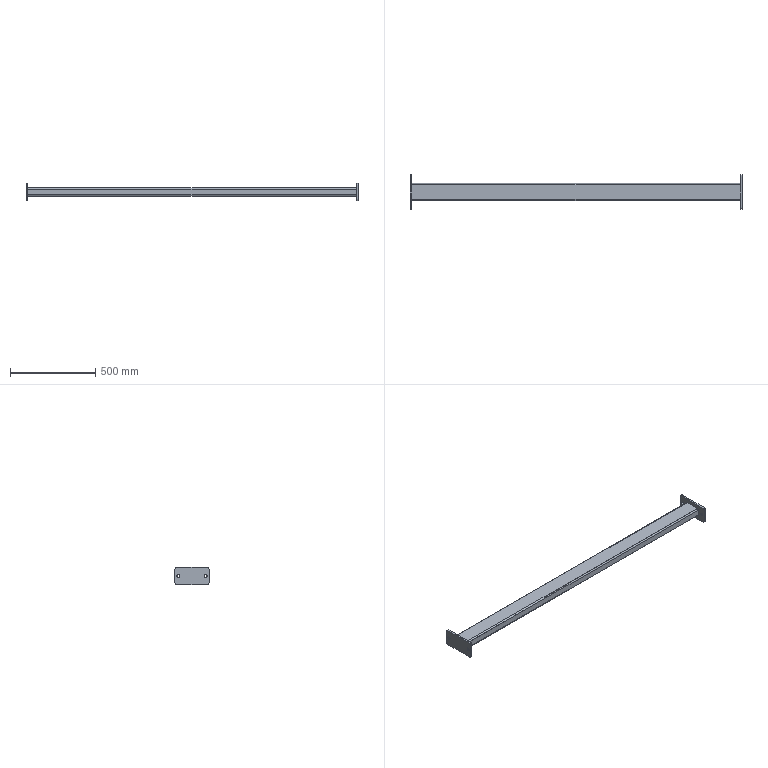Part | SolidWorks | features Fillet 1, HoleWzd 1, ICE 1, MirrorSolid 1, WeldMemberFeat 1, WeldmentFeature 1 | 3 solids | 46 faces | box 1950 x 200 x 100 mm | volume 2501619 mm3 | cylinder 24 | plane 22 | commonest cylinder face diameters 17.5 x8 20 x8 8 x4 16 x4
STEP:
#1=CARTESIAN_POINT('',(-965.,42.,-25.));
#2=VERTEX_POINT('',#1);
#3=CARTESIAN_POINT('',(-965.,50.,-17.));
#4=VERTEX_POINT('',#3);
#5=CARTESIAN_POINT('',(-965.,42.,-17.));
#6=DIRECTION('',(1.,0.,0.));
#7=DIRECTION('',(0.,0.,-1.));
#8=AXIS2_PLACEMENT_3D('',#5,#6,#7);
#9=CIRCLE('',#8,8.);
#10=EDGE_CURVE('',#2,#4,#9,.T.);
#11=ORIENTED_EDGE('',*,*,#10,.T.);
#12=CARTESIAN_POINT('',(965.,50.,-17.));
#13=VERTEX_POINT('',#12);
#14=CARTESIAN_POINT('',(965.,50.,-17.));
#15=DIRECTION('',(-1.,0.,0.));
#16=VECTOR('',#15,1000.);
#17=LINE('',#14,#16);
#18=EDGE_CURVE('',#13,#4,#17,.T.);
#19=ORIENTED_EDGE('',*,*,#18,.F.);
#20=CARTESIAN_POINT('',(965.,42.,-25.));
#21=VERTEX_POINT('',#20);
#22=CARTESIAN_POINT('',(965.,42.,-17.));
#23=DIRECTION('',(1.,0.,0.));
#24=DIRECTION('',(0.,0.,-1.));
#25=AXIS2_PLACEMENT_3D('',#22,#23,#24);
#26=CIRCLE('',#25,8.);
#27=EDGE_CURVE('',#21,#13,#26,.T.);
#28=ORIENTED_EDGE('',*,*,#27,.F.);
#29=CARTESIAN_POINT('',(965.,42.,-25.));
#30=DIRECTION('',(-1.,0.,0.));
#31=VECTOR('',#30,1000.);
#32=LINE('',#29,#31);
#33=EDGE_CURVE('',#21,#2,#32,.T.);
#34=ORIENTED_EDGE('',*,*,#33,.T.);
#35=EDGE_LOOP('',(#11,#19,#28,#34));
#36=FACE_OUTER_BOUND('',#35,.T.);
#37=CARTESIAN_POINT('',(965.,42.,-17.));
#38=DIRECTION('',(-1.,0.,0.));
#39=DIRECTION('',(0.,0.,1.));
#40=AXIS2_PLACEMENT_3D('',#37,#38,#39);
#41=CYLINDRICAL_SURFACE('',#40,8.);
#42=ADVANCED_FACE('',(#36),#41,.T.);
#43=CARTESIAN_POINT('',(-965.,50.,17.));
#44=VERTEX_POINT('',#43);
#45=CARTESIAN_POINT('',(-965.,50.,-17.));
#46=DIRECTION('',(0.,0.,1.));
#47=VECTOR('',#46,1000.);
#48=LINE('',#45,#47);
#49=EDGE_CURVE('',#4,#44,#48,.T.);
#50=ORIENTED_EDGE('',*,*,#49,.T.);
#51=CARTESIAN_POINT('',(965.,50.,17.));
#52=VERTEX_POINT('',#51);
#53=CARTESIAN_POINT('',(965.,50.,17.));
#54=DIRECTION('',(-1.,0.,0.));
#55=VECTOR('',#54,1000.);
#56=LINE('',#53,#55);
#57=EDGE_CURVE('',#52,#44,#56,.T.);
#58=ORIENTED_EDGE('',*,*,#57,.F.);
#59=CARTESIAN_POINT('',(965.,50.,-17.));
#60=DIRECTION('',(0.,0.,1.));
#61=VECTOR('',#60,1000.);
#62=LINE('',#59,#61);
#63=EDGE_CURVE('',#13,#52,#62,.T.);
#64=ORIENTED_EDGE('',*,*,#63,.F.);
#65=ORIENTED_EDGE('',*,*,#18,.T.);
#66=EDGE_LOOP('',(#50,#58,#64,#65));
#67=FACE_OUTER_BOUND('',#66,.T.);
#68=CARTESIAN_POINT('',(965.,50.,-17.));
#69=DIRECTION('',(0.,-1.,0.));
#70=DIRECTION('',(0.,0.,-1.));
#71=AXIS2_PLACEMENT_3D('',#68,#69,#70);
#72=PLANE('',#71);
#73=ADVANCED_FACE('',(#67),#72,.F.);
#74=CARTESIAN_POINT('',(-965.,42.,25.));
#75=VERTEX_POINT('',#74);
#76=CARTESIAN_POINT('',(-965.,42.,17.));
#77=DIRECTION('',(1.,0.,0.));
#78=DIRECTION('',(0.,0.,-1.));
#79=AXIS2_PLACEMENT_3D('',#76,#77,#78);
#80=CIRCLE('',#79,8.);
#81=EDGE_CURVE('',#44,#75,#80,.T.);
#82=ORIENTED_EDGE('',*,*,#81,.T.);
#83=CARTESIAN_POINT('',(965.,42.,25.));
#84=VERTEX_POINT('',#83);
#85=CARTESIAN_POINT('',(965.,42.,25.));
#86=DIRECTION('',(-1.,0.,0.));
#87=VECTOR('',#86,1000.);
#88=LINE('',#85,#87);
#89=EDGE_CURVE('',#84,#75,#88,.T.);
#90=ORIENTED_EDGE('',*,*,#89,.F.);
#91=CARTESIAN_POINT('',(965.,42.,17.));
#92=DIRECTION('',(1.,0.,0.));
#93=DIRECTION('',(0.,0.,-1.));
#94=AXIS2_PLACEMENT_3D('',#91,#92,#93);
#95=CIRCLE('',#94,8.);
#96=EDGE_CURVE('',#52,#84,#95,.T.);
#97=ORIENTED_EDGE('',*,*,#96,.F.);
#98=ORIENTED_EDGE('',*,*,#57,.T.);
#99=EDGE_LOOP('',(#82,#90,#97,#98));
#100=FACE_OUTER_BOUND('',#99,.T.);
#101=CARTESIAN_POINT('',(965.,42.,17.));
#102=DIRECTION('',(-1.,0.,0.));
#103=DIRECTION('',(0.,0.,1.));
#104=AXIS2_PLACEMENT_3D('',#101,#102,#103);
#105=CYLINDRICAL_SURFACE('',#104,8.);
#106=ADVANCED_FACE('',(#100),#105,.T.);
#107=CARTESIAN_POINT('',(-965.,-42.,25.));
#108=VERTEX_POINT('',#107);
#109=CARTESIAN_POINT('',(-965.,-42.,25.));
#110=DIRECTION('',(0.,-1.,0.));
#111=VECTOR('',#110,1000.);
#112=LINE('',#109,#111);
#113=EDGE_CURVE('',#75,#108,#112,.T.);
#114=ORIENTED_EDGE('',*,*,#113,.T.);
#115=CARTESIAN_POINT('',(965.,-42.,25.));
#116=VERTEX_POINT('',#115);
#117=CARTESIAN_POINT('',(965.,-42.,25.));
#118=DIRECTION('',(-1.,0.,0.));
#119=VECTOR('',#118,1000.);
#120=LINE('',#117,#119);
#121=EDGE_CURVE('',#116,#108,#120,.T.);
#122=ORIENTED_EDGE('',*,*,#121,.F.);
#123=CARTESIAN_POINT('',(965.,-42.,25.));
#124=DIRECTION('',(0.,-1.,0.));
#125=VECTOR('',#124,1000.);
#126=LINE('',#123,#125);
#127=EDGE_CURVE('',#84,#116,#126,.T.);
#128=ORIENTED_EDGE('',*,*,#127,.F.);
#129=ORIENTED_EDGE('',*,*,#89,.T.);
#130=EDGE_LOOP('',(#114,#122,#128,#129));
#131=FACE_OUTER_BOUND('',#130,.T.);
#132=CARTESIAN_POINT('',(965.,-42.,25.));
#133=DIRECTION('',(0.,0.,-1.));
#134=DIRECTION('',(-1.,0.,0.));
#135=AXIS2_PLACEMENT_3D('',#132,#133,#134);
#136=PLANE('',#135);
#137=ADVANCED_FACE('',(#131),#136,.F.);
#138=CARTESIAN_POINT('',(-965.,-50.,17.));
#139=VERTEX_POINT('',#138);
#140=CARTESIAN_POINT('',(-965.,-42.,17.));
#141=DIRECTION('',(1.,0.,0.));
#142=DIRECTION('',(0.,0.,-1.));
#143=AXIS2_PLACEMENT_3D('',#140,#141,#142);
#144=CIRCLE('',#143,8.);
#145=EDGE_CURVE('',#108,#139,#144,.T.);
#146=ORIENTED_EDGE('',*,*,#145,.T.);
#147=CARTESIAN_POINT('',(965.,-50.,17.));
#148=VERTEX_POINT('',#147);
#149=CARTESIAN_POINT('',(965.,-50.,17.));
#150=DIRECTION('',(-1.,0.,0.));
#151=VECTOR('',#150,1000.);
#152=LINE('',#149,#151);
#153=EDGE_CURVE('',#148,#139,#152,.T.);
#154=ORIENTED_EDGE('',*,*,#153,.F.);
#155=CARTESIAN_POINT('',(965.,-42.,17.));
#156=DIRECTION('',(1.,0.,0.));
#157=DIRECTION('',(0.,0.,-1.));
#158=AXIS2_PLACEMENT_3D('',#155,#156,#157);
#159=CIRCLE('',#158,8.);
#160=EDGE_CURVE('',#116,#148,#159,.T.);
#161=ORIENTED_EDGE('',*,*,#160,.F.);
#162=ORIENTED_EDGE('',*,*,#121,.T.);
#163=EDGE_LOOP('',(#146,#154,#161,#162));
#164=FACE_OUTER_BOUND('',#163,.T.);
#165=CARTESIAN_POINT('',(965.,-42.,17.));
#166=DIRECTION('',(-1.,0.,0.));
#167=DIRECTION('',(0.,0.,1.));
#168=AXIS2_PLACEMENT_3D('',#165,#166,#167);
#169=CYLINDRICAL_SURFACE('',#168,8.);
#170=ADVANCED_FACE('',(#164),#169,.T.);
#171=CARTESIAN_POINT('',(-965.,-50.,-17.));
#172=VERTEX_POINT('',#171);
#173=CARTESIAN_POINT('',(-965.,-50.,17.));
#174=DIRECTION('',(0.,0.,-1.));
#175=VECTOR('',#174,1000.);
#176=LINE('',#173,#175);
#177=EDGE_CURVE('',#139,#172,#176,.T.);
#178=ORIENTED_EDGE('',*,*,#177,.T.);
#179=CARTESIAN_POINT('',(965.,-50.,-17.));
#180=VERTEX_POINT('',#179);
#181=CARTESIAN_POINT('',(965.,-50.,-17.));
#182=DIRECTION('',(-1.,0.,0.));
#183=VECTOR('',#182,1000.);
#184=LINE('',#181,#183);
#185=EDGE_CURVE('',#180,#172,#184,.T.);
#186=ORIENTED_EDGE('',*,*,#185,.F.);
#187=CARTESIAN_POINT('',(965.,-50.,17.));
#188=DIRECTION('',(0.,0.,-1.));
#189=VECTOR('',#188,1000.);
#190=LINE('',#187,#189);
#191=EDGE_CURVE('',#148,#180,#190,.T.);
#192=ORIENTED_EDGE('',*,*,#191,.F.);
#193=ORIENTED_EDGE('',*,*,#153,.T.);
#194=EDGE_LOOP('',(#178,#186,#192,#193));
#195=FACE_OUTER_BOUND('',#194,.T.);
#196=CARTESIAN_POINT('',(965.,-50.,17.));
#197=DIRECTION('',(0.,1.,0.));
#198=DIRECTION('',(0.,0.,1.));
#199=AXIS2_PLACEMENT_3D('',#196,#197,#198);
#200=PLANE('',#199);
#201=ADVANCED_FACE('',(#195),#200,.F.);
#202=CARTESIAN_POINT('',(-965.,-42.,-25.));
#203=VERTEX_POINT('',#202);
#204=CARTESIAN_POINT('',(-965.,-42.,-17.));
#205=DIRECTION('',(1.,0.,0.));
#206=DIRECTION('',(0.,0.,-1.));
#207=AXIS2_PLACEMENT_3D('',#204,#205,#206);
#208=CIRCLE('',#207,8.);
#209=EDGE_CURVE('',#172,#203,#208,.T.);
#210=ORIENTED_EDGE('',*,*,#209,.T.);
#211=CARTESIAN_POINT('',(965.,-42.,-25.));
#212=VERTEX_POINT('',#211);
#213=CARTESIAN_POINT('',(965.,-42.,-25.));
#214=DIRECTION('',(-1.,0.,0.));
#215=VECTOR('',#214,1000.);
#216=LINE('',#213,#215);
#217=EDGE_CURVE('',#212,#203,#216,.T.);
#218=ORIENTED_EDGE('',*,*,#217,.F.);
#219=CARTESIAN_POINT('',(965.,-42.,-17.));
#220=DIRECTION('',(1.,0.,0.));
#221=DIRECTION('',(0.,0.,-1.));
#222=AXIS2_PLACEMENT_3D('',#219,#220,#221);
#223=CIRCLE('',#222,8.);
#224=EDGE_CURVE('',#180,#212,#223,.T.);
#225=ORIENTED_EDGE('',*,*,#224,.F.);
#226=ORIENTED_EDGE('',*,*,#185,.T.);
#227=EDGE_LOOP('',(#210,#218,#225,#226));
#228=FACE_OUTER_BOUND('',#227,.T.);
#229=CARTESIAN_POINT('',(965.,-42.,-17.));
#230=DIRECTION('',(-1.,0.,0.));
#231=DIRECTION('',(0.,0.,1.));
#232=AXIS2_PLACEMENT_3D('',#229,#230,#231);
#233=CYLINDRICAL_SURFACE('',#232,8.);
#234=ADVANCED_FACE('',(#228),#233,.T.);
#235=CARTESIAN_POINT('',(-965.,46.,17.));
#236=VERTEX_POINT('',#235);
#237=CARTESIAN_POINT('',(-965.,42.,21.));
#238=VERTEX_POINT('',#237);
#239=CARTESIAN_POINT('',(-965.,42.,17.));
#240=DIRECTION('',(1.,0.,0.));
#241=DIRECTION('',(0.,0.,-1.));
#242=AXIS2_PLACEMENT_3D('',#239,#240,#241);
#243=CIRCLE('',#242,4.);
#244=EDGE_CURVE('',#236,#238,#243,.T.);
#245=ORIENTED_EDGE('',*,*,#244,.F.);
#246=CARTESIAN_POINT('',(965.,46.,17.));
#247=VERTEX_POINT('',#246);
#248=CARTESIAN_POINT('',(965.,46.,17.));
#249=DIRECTION('',(-1.,0.,0.));
#250=VECTOR('',#249,1000.);
#251=LINE('',#248,#250);
#252=EDGE_CURVE('',#247,#236,#251,.T.);
#253=ORIENTED_EDGE('',*,*,#252,.F.);
#254=CARTESIAN_POINT('',(965.,42.,21.));
#255=VERTEX_POINT('',#254);
#256=CARTESIAN_POINT('',(965.,42.,17.));
#257=DIRECTION('',(1.,0.,0.));
#258=DIRECTION('',(0.,0.,-1.));
#259=AXIS2_PLACEMENT_3D('',#256,#257,#258);
#260=CIRCLE('',#259,4.);
#261=EDGE_CURVE('',#247,#255,#260,.T.);
#262=ORIENTED_EDGE('',*,*,#261,.T.);
#263=CARTESIAN_POINT('',(965.,42.,21.));
#264=DIRECTION('',(-1.,0.,0.));
#265=VECTOR('',#264,1000.);
#266=LINE('',#263,#265);
#267=EDGE_CURVE('',#255,#238,#266,.T.);
#268=ORIENTED_EDGE('',*,*,#267,.T.);
#269=EDGE_LOOP('',(#245,#253,#262,#268));
#270=FACE_OUTER_BOUND('',#269,.T.);
#271=CARTESIAN_POINT('',(965.,42.,17.));
#272=DIRECTION('',(-1.,0.,0.));
#273=DIRECTION('',(0.,0.,1.));
#274=AXIS2_PLACEMENT_3D('',#271,#272,#273);
#275=CYLINDRICAL_SURFACE('',#274,4.);
#276=ADVANCED_FACE('',(#270),#275,.F.);
#277=CARTESIAN_POINT('',(-965.,46.,-17.));
#278=VERTEX_POINT('',#277);
#279=CARTESIAN_POINT('',(-965.,46.,-17.));
#280=DIRECTION('',(0.,0.,1.));
#281=VECTOR('',#280,1000.);
#282=LINE('',#279,#281);
#283=EDGE_CURVE('',#278,#236,#282,.T.);
#284=ORIENTED_EDGE('',*,*,#283,.F.);
#285=CARTESIAN_POINT('',(965.,46.,-17.));
#286=VERTEX_POINT('',#285);
#287=CARTESIAN_POINT('',(965.,46.,-17.));
#288=DIRECTION('',(-1.,0.,0.));
#289=VECTOR('',#288,1000.);
#290=LINE('',#287,#289);
#291=EDGE_CURVE('',#286,#278,#290,.T.);
#292=ORIENTED_EDGE('',*,*,#291,.F.);
#293=CARTESIAN_POINT('',(965.,46.,-17.));
#294=DIRECTION('',(0.,0.,1.));
#295=VECTOR('',#294,1000.);
#296=LINE('',#293,#295);
#297=EDGE_CURVE('',#286,#247,#296,.T.);
#298=ORIENTED_EDGE('',*,*,#297,.T.);
#299=ORIENTED_EDGE('',*,*,#252,.T.);
#300=EDGE_LOOP('',(#284,#292,#298,#299));
#301=FACE_OUTER_BOUND('',#300,.T.);
#302=CARTESIAN_POINT('',(965.,46.,-17.));
#303=DIRECTION('',(0.,-1.,0.));
#304=DIRECTION('',(0.,0.,-1.));
#305=AXIS2_PLACEMENT_3D('',#302,#303,#304);
#306=PLANE('',#305);
#307=ADVANCED_FACE('',(#301),#306,.T.);
#308=CARTESIAN_POINT('',(-965.,42.,-21.));
#309=VERTEX_POINT('',#308);
#310=CARTESIAN_POINT('',(-965.,42.,-17.));
#311=DIRECTION('',(1.,0.,0.));
#312=DIRECTION('',(0.,0.,-1.));
#313=AXIS2_PLACEMENT_3D('',#310,#311,#312);
#314=CIRCLE('',#313,4.);
#315=EDGE_CURVE('',#309,#278,#314,.T.);
#316=ORIENTED_EDGE('',*,*,#315,.F.);
#317=CARTESIAN_POINT('',(965.,42.,-21.));
#318=VERTEX_POINT('',#317);
#319=CARTESIAN_POINT('',(965.,42.,-21.));
#320=DIRECTION('',(-1.,0.,0.));
#321=VECTOR('',#320,1000.);
#322=LINE('',#319,#321);
#323=EDGE_CURVE('',#318,#309,#322,.T.);
#324=ORIENTED_EDGE('',*,*,#323,.F.);
#325=CARTESIAN_POINT('',(965.,42.,-17.));
#326=DIRECTION('',(1.,0.,0.));
#327=DIRECTION('',(0.,0.,-1.));
#328=AXIS2_PLACEMENT_3D('',#325,#326,#327);
#329=CIRCLE('',#328,4.);
#330=EDGE_CURVE('',#318,#286,#329,.T.);
#331=ORIENTED_EDGE('',*,*,#330,.T.);
#332=ORIENTED_EDGE('',*,*,#291,.T.);
#333=EDGE_LOOP('',(#316,#324,#331,#332));
#334=FACE_OUTER_BOUND('',#333,.T.);
#335=CARTESIAN_POINT('',(965.,42.,-17.));
#336=DIRECTION('',(-1.,0.,0.));
#337=DIRECTION('',(0.,0.,1.));
#338=AXIS2_PLACEMENT_3D('',#335,#336,#337);
#339=CYLINDRICAL_SURFACE('',#338,4.);
#340=ADVANCED_FACE('',(#334),#339,.F.);
#341=CARTESIAN_POINT('',(-965.,-42.,-21.));
#342=VERTEX_POINT('',#341);
#343=CARTESIAN_POINT('',(-965.,42.,-21.));
#344=DIRECTION('',(0.,1.,0.));
#345=VECTOR('',#344,1000.);
#346=LINE('',#343,#345);
#347=EDGE_CURVE('',#342,#309,#346,.T.);
#348=ORIENTED_EDGE('',*,*,#347,.F.);
#349=CARTESIAN_POINT('',(965.,-42.,-21.));
#350=VERTEX_POINT('',#349);
#351=CARTESIAN_POINT('',(965.,-42.,-21.));
#352=DIRECTION('',(-1.,0.,0.));
#353=VECTOR('',#352,1000.);
#354=LINE('',#351,#353);
#355=EDGE_CURVE('',#350,#342,#354,.T.);
#356=ORIENTED_EDGE('',*,*,#355,.F.);
#357=CARTESIAN_POINT('',(965.,42.,-21.));
#358=DIRECTION('',(0.,1.,0.));
#359=VECTOR('',#358,1000.);
#360=LINE('',#357,#359);
#361=EDGE_CURVE('',#350,#318,#360,.T.);
#362=ORIENTED_EDGE('',*,*,#361,.T.);
#363=ORIENTED_EDGE('',*,*,#323,.T.);
#364=EDGE_LOOP('',(#348,#356,#362,#363));
#365=FACE_OUTER_BOUND('',#364,.T.);
#366=CARTESIAN_POINT('',(965.,42.,-21.));
#367=DIRECTION('',(0.,0.,1.));
#368=DIRECTION('',(1.,0.,0.));
#369=AXIS2_PLACEMENT_3D('',#366,#367,#368);
#370=PLANE('',#369);
#371=ADVANCED_FACE('',(#365),#370,.T.);
#372=CARTESIAN_POINT('',(-965.,-46.,-17.));
#373=VERTEX_POINT('',#372);
#374=CARTESIAN_POINT('',(-965.,-42.,-17.));
#375=DIRECTION('',(1.,0.,0.));
#376=DIRECTION('',(0.,0.,-1.));
#377=AXIS2_PLACEMENT_3D('',#374,#375,#376);
#378=CIRCLE('',#377,4.);
#379=EDGE_CURVE('',#373,#342,#378,.T.);
#380=ORIENTED_EDGE('',*,*,#379,.F.);
#381=CARTESIAN_POINT('',(965.,-46.,-17.));
#382=VERTEX_POINT('',#381);
#383=CARTESIAN_POINT('',(965.,-46.,-17.));
#384=DIRECTION('',(-1.,0.,0.));
#385=VECTOR('',#384,1000.);
#386=LINE('',#383,#385);
#387=EDGE_CURVE('',#382,#373,#386,.T.);
#388=ORIENTED_EDGE('',*,*,#387,.F.);
#389=CARTESIAN_POINT('',(965.,-42.,-17.));
#390=DIRECTION('',(1.,0.,0.));
#391=DIRECTION('',(0.,0.,-1.));
#392=AXIS2_PLACEMENT_3D('',#389,#390,#391);
#393=CIRCLE('',#392,4.);
#394=EDGE_CURVE('',#382,#350,#393,.T.);
#395=ORIENTED_EDGE('',*,*,#394,.T.);
#396=ORIENTED_EDGE('',*,*,#355,.T.);
#397=EDGE_LOOP('',(#380,#388,#395,#396));
#398=FACE_OUTER_BOUND('',#397,.T.);
#399=CARTESIAN_POINT('',(965.,-42.,-17.));
#400=DIRECTION('',(-1.,0.,0.));
#401=DIRECTION('',(0.,0.,1.));
#402=AXIS2_PLACEMENT_3D('',#399,#400,#401);
#403=CYLINDRICAL_SURFACE('',#402,4.);
#404=ADVANCED_FACE('',(#398),#403,.F.);
#405=CARTESIAN_POINT('',(-965.,-46.,17.));
#406=VERTEX_POINT('',#405);
#407=CARTESIAN_POINT('',(-965.,-46.,17.));
#408=DIRECTION('',(0.,0.,-1.));
#409=VECTOR('',#408,1000.);
#410=LINE('',#407,#409);
#411=EDGE_CURVE('',#406,#373,#410,.T.);
#412=ORIENTED_EDGE('',*,*,#411,.F.);
#413=CARTESIAN_POINT('',(965.,-46.,17.));
#414=VERTEX_POINT('',#413);
#415=CARTESIAN_POINT('',(965.,-46.,17.));
#416=DIRECTION('',(-1.,0.,0.));
#417=VECTOR('',#416,1000.);
#418=LINE('',#415,#417);
#419=EDGE_CURVE('',#414,#406,#418,.T.);
#420=ORIENTED_EDGE('',*,*,#419,.F.);
#421=CARTESIAN_POINT('',(965.,-46.,17.));
#422=DIRECTION('',(0.,0.,-1.));
#423=VECTOR('',#422,1000.);
#424=LINE('',#421,#423);
#425=EDGE_CURVE('',#414,#382,#424,.T.);
#426=ORIENTED_EDGE('',*,*,#425,.T.);
#427=ORIENTED_EDGE('',*,*,#387,.T.);
#428=EDGE_LOOP('',(#412,#420,#426,#427));
#429=FACE_OUTER_BOUND('',#428,.T.);
#430=CARTESIAN_POINT('',(965.,-46.,17.));
#431=DIRECTION('',(0.,1.,0.));
#432=DIRECTION('',(0.,0.,1.));
#433=AXIS2_PLACEMENT_3D('',#430,#431,#432);
#434=PLANE('',#433);
#435=ADVANCED_FACE('',(#429),#434,.T.);
#436=CARTESIAN_POINT('',(-965.,-42.,21.));
#437=VERTEX_POINT('',#436);
#438=CARTESIAN_POINT('',(-965.,-42.,17.));
#439=DIRECTION('',(1.,0.,0.));
#440=DIRECTION('',(0.,0.,-1.));
#441=AXIS2_PLACEMENT_3D('',#438,#439,#440);
#442=CIRCLE('',#441,4.);
#443=EDGE_CURVE('',#437,#406,#442,.T.);
#444=ORIENTED_EDGE('',*,*,#443,.F.);
#445=CARTESIAN_POINT('',(965.,-42.,21.));
#446=VERTEX_POINT('',#445);
#447=CARTESIAN_POINT('',(965.,-42.,21.));
#448=DIRECTION('',(-1.,0.,0.));
#449=VECTOR('',#448,1000.);
#450=LINE('',#447,#449);
#451=EDGE_CURVE('',#446,#437,#450,.T.);
#452=ORIENTED_EDGE('',*,*,#451,.F.);
#453=CARTESIAN_POINT('',(965.,-42.,17.));
#454=DIRECTION('',(1.,0.,0.));
#455=DIRECTION('',(0.,0.,-1.));
#456=AXIS2_PLACEMENT_3D('',#453,#454,#455);
#457=CIRCLE('',#456,4.);
#458=EDGE_CURVE('',#446,#414,#457,.T.);
#459=ORIENTED_EDGE('',*,*,#458,.T.);
#460=ORIENTED_EDGE('',*,*,#419,.T.);
#461=EDGE_LOOP('',(#444,#452,#459,#460));
#462=FACE_OUTER_BOUND('',#461,.T.);
#463=CARTESIAN_POINT('',(965.,-42.,17.));
#464=DIRECTION('',(-1.,0.,0.));
#465=DIRECTION('',(0.,0.,1.));
#466=AXIS2_PLACEMENT_3D('',#463,#464,#465);
#467=CYLINDRICAL_SURFACE('',#466,4.);
#468=ADVANCED_FACE('',(#462),#467,.F.);
#469=CARTESIAN_POINT('',(-965.,-42.,21.));
#470=DIRECTION('',(0.,-1.,0.));
#471=VECTOR('',#470,1000.);
#472=LINE('',#469,#471);
#473=EDGE_CURVE('',#238,#437,#472,.T.);
#474=ORIENTED_EDGE('',*,*,#473,.F.);
#475=ORIENTED_EDGE('',*,*,#267,.F.);
#476=CARTESIAN_POINT('',(965.,-42.,21.));
#477=DIRECTION('',(0.,-1.,0.));
#478=VECTOR('',#477,1000.);
#479=LINE('',#476,#478);
#480=EDGE_CURVE('',#255,#446,#479,.T.);
#481=ORIENTED_EDGE('',*,*,#480,.T.);
#482=ORIENTED_EDGE('',*,*,#451,.T.);
#483=EDGE_LOOP('',(#474,#475,#481,#482));
#484=FACE_OUTER_BOUND('',#483,.T.);
#485=CARTESIAN_POINT('',(965.,-42.,21.));
#486=DIRECTION('',(0.,0.,-1.));
#487=DIRECTION('',(-1.,0.,0.));
#488=AXIS2_PLACEMENT_3D('',#485,#486,#487);
#489=PLANE('',#488);
#490=ADVANCED_FACE('',(#484),#489,.T.);
#491=CARTESIAN_POINT('',(-965.,42.,-25.));
#492=DIRECTION('',(0.,1.,0.));
#493=VECTOR('',#492,1000.);
#494=LINE('',#491,#493);
#495=EDGE_CURVE('',#203,#2,#494,.T.);
#496=ORIENTED_EDGE('',*,*,#495,.T.);
#497=ORIENTED_EDGE('',*,*,#33,.F.);
#498=CARTESIAN_POINT('',(965.,42.,-25.));
#499=DIRECTION('',(0.,1.,0.));
#500=VECTOR('',#499,1000.);
#501=LINE('',#498,#500);
#502=EDGE_CURVE('',#212,#21,#501,.T.);
#503=ORIENTED_EDGE('',*,*,#502,.F.);
#504=ORIENTED_EDGE('',*,*,#217,.T.);
#505=EDGE_LOOP('',(#496,#497,#503,#504));
#506=FACE_OUTER_BOUND('',#505,.T.);
#507=CARTESIAN_POINT('',(965.,42.,-25.));
#508=DIRECTION('',(0.,0.,1.));
#509=DIRECTION('',(1.,0.,0.));
#510=AXIS2_PLACEMENT_3D('',#507,#508,#509);
#511=PLANE('',#510);
#512=ADVANCED_FACE('',(#506),#511,.F.);
#513=ORIENTED_EDGE('',*,*,#261,.F.);
#514=ORIENTED_EDGE('',*,*,#297,.F.);
#515=ORIENTED_EDGE('',*,*,#330,.F.);
#516=ORIENTED_EDGE('',*,*,#361,.F.);
#517=ORIENTED_EDGE('',*,*,#394,.F.);
#518=ORIENTED_EDGE('',*,*,#425,.F.);
#519=ORIENTED_EDGE('',*,*,#458,.F.);
#520=ORIENTED_EDGE('',*,*,#480,.F.);
#521=EDGE_LOOP('',(#513,#514,#515,#516,#517,#518,#519,#520));
#522=FACE_BOUND('',#521,.T.);
#523=ORIENTED_EDGE('',*,*,#27,.T.);
#524=ORIENTED_EDGE('',*,*,#63,.T.);
#525=ORIENTED_EDGE('',*,*,#96,.T.);
#526=ORIENTED_EDGE('',*,*,#127,.T.);
#527=ORIENTED_EDGE('',*,*,#160,.T.);
#528=ORIENTED_EDGE('',*,*,#191,.T.);
#529=ORIENTED_EDGE('',*,*,#224,.T.);
#530=ORIENTED_EDGE('',*,*,#502,.T.);
#531=EDGE_LOOP('',(#523,#524,#525,#526,#527,#528,#529,#530));
#532=FACE_OUTER_BOUND('',#531,.T.);
#533=CARTESIAN_POINT('',(965.,42.,-17.));
#534=DIRECTION('',(1.,0.,0.));
#535=DIRECTION('',(0.,0.,-1.));
#536=AXIS2_PLACEMENT_3D('',#533,#534,#535);
#537=PLANE('',#536);
#538=ADVANCED_FACE('',(#522,#532),#537,.T.);
#539=ORIENTED_EDGE('',*,*,#244,.T.);
#540=ORIENTED_EDGE('',*,*,#473,.T.);
#541=ORIENTED_EDGE('',*,*,#443,.T.);
#542=ORIENTED_EDGE('',*,*,#411,.T.);
#543=ORIENTED_EDGE('',*,*,#379,.T.);
#544=ORIENTED_EDGE('',*,*,#347,.T.);
#545=ORIENTED_EDGE('',*,*,#315,.T.);
#546=ORIENTED_EDGE('',*,*,#283,.T.);
#547=EDGE_LOOP('',(#539,#540,#541,#542,#543,#544,#545,#546));
#548=FACE_BOUND('',#547,.T.);
#549=ORIENTED_EDGE('',*,*,#10,.F.);
#550=ORIENTED_EDGE('',*,*,#495,.F.);
#551=ORIENTED_EDGE('',*,*,#209,.F.);
#552=ORIENTED_EDGE('',*,*,#177,.F.);
#553=ORIENTED_EDGE('',*,*,#145,.F.);
#554=ORIENTED_EDGE('',*,*,#113,.F.);
#555=ORIENTED_EDGE('',*,*,#81,.F.);
#556=ORIENTED_EDGE('',*,*,#49,.F.);
#557=EDGE_LOOP('',(#549,#550,#551,#552,#553,#554,#555,#556));
#558=FACE_OUTER_BOUND('',#557,.T.);
#559=CARTESIAN_POINT('',(-965.,42.,-17.));
#560=DIRECTION('',(1.,0.,0.));
#561=DIRECTION('',(0.,0.,-1.));
#562=AXIS2_PLACEMENT_3D('',#559,#560,#561);
#563=PLANE('',#562);
#564=ADVANCED_FACE('',(#548,#558),#563,.F.);
#565=CLOSED_SHELL('',(#42,#73,#106,#137,#170,#201,#234,#276,#307,#340,#371,#404,#435,#468,#490,#512,#538,#564));
#566=MANIFOLD_SOLID_BREP('',#565);
#567=CARTESIAN_POINT('',(-965.,80.,8.75));
#568=VERTEX_POINT('',#567);
#569=CARTESIAN_POINT('',(-965.,80.,-8.75));
#570=VERTEX_POINT('',#569);
#571=CARTESIAN_POINT('',(-965.,80.,0.));
#572=DIRECTION('',(1.,0.,0.));
#573=DIRECTION('',(0.,0.,-1.));
#574=AXIS2_PLACEMENT_3D('',#571,#572,#573);
#575=CIRCLE('',#574,8.75);
#576=EDGE_CURVE('',#568,#570,#575,.T.);
#577=ORIENTED_EDGE('',*,*,#576,.T.);
#578=CARTESIAN_POINT('',(-975.,80.,-8.75));
#579=VERTEX_POINT('',#578);
#580=CARTESIAN_POINT('',(-975.,80.,-8.75));
#581=DIRECTION('',(-1.,0.,0.));
#582=VECTOR('',#581,1000.);
#583=LINE('',#580,#582);
#584=EDGE_CURVE('',#570,#579,#583,.T.);
#585=ORIENTED_EDGE('',*,*,#584,.T.);
#586=CARTESIAN_POINT('',(-975.,80.,8.75));
#587=VERTEX_POINT('',#586);
#588=CARTESIAN_POINT('',(-975.,80.,0.));
#589=DIRECTION('',(-1.,0.,0.));
#590=DIRECTION('',(0.,0.,1.));
#591=AXIS2_PLACEMENT_3D('',#588,#589,#590);
#592=CIRCLE('',#591,8.75);
#593=EDGE_CURVE('',#579,#587,#592,.T.);
#594=ORIENTED_EDGE('',*,*,#593,.T.);
#595=CARTESIAN_POINT('',(-975.,80.,8.75));
#596=DIRECTION('',(-1.,0.,0.));
#597=VECTOR('',#596,1000.);
#598=LINE('',#595,#597);
#599=EDGE_CURVE('',#568,#587,#598,.T.);
#600=ORIENTED_EDGE('',*,*,#599,.F.);
#601=EDGE_LOOP('',(#577,#585,#594,#600));
#602=FACE_OUTER_BOUND('',#601,.T.);
#603=CARTESIAN_POINT('',(-975.,80.,0.));
#604=DIRECTION('',(-1.,0.,0.));
#605=DIRECTION('',(0.,0.,1.));
#606=AXIS2_PLACEMENT_3D('',#603,#604,#605);
#607=CYLINDRICAL_SURFACE('',#606,8.75);
#608=ADVANCED_FACE('',(#602),#607,.F.);
#609=CARTESIAN_POINT('',(-965.,-80.,8.75));
#610=VERTEX_POINT('',#609);
#611=CARTESIAN_POINT('',(-965.,-80.,-8.75));
#612=VERTEX_POINT('',#611);
#613=CARTESIAN_POINT('',(-965.,-80.,0.));
#614=DIRECTION('',(1.,0.,0.));
#615=DIRECTION('',(0.,0.,-1.));
#616=AXIS2_PLACEMENT_3D('',#613,#614,#615);
#617=CIRCLE('',#616,8.75);
#618=EDGE_CURVE('',#610,#612,#617,.T.);
#619=ORIENTED_EDGE('',*,*,#618,.T.);
#620=CARTESIAN_POINT('',(-975.,-80.,-8.75));
#621=VERTEX_POINT('',#620);
#622=CARTESIAN_POINT('',(-975.,-80.,-8.75));
#623=DIRECTION('',(-1.,0.,0.));
#624=VECTOR('',#623,1000.);
#625=LINE('',#622,#624);
#626=EDGE_CURVE('',#612,#621,#625,.T.);
#627=ORIENTED_EDGE('',*,*,#626,.T.);
#628=CARTESIAN_POINT('',(-975.,-80.,8.75));
#629=VERTEX_POINT('',#628);
#630=CARTESIAN_POINT('',(-975.,-80.,0.));
#631=DIRECTION('',(-1.,0.,0.));
#632=DIRECTION('',(0.,0.,1.));
#633=AXIS2_PLACEMENT_3D('',#630,#631,#632);
#634=CIRCLE('',#633,8.75);
#635=EDGE_CURVE('',#621,#629,#634,.T.);
#636=ORIENTED_EDGE('',*,*,#635,.T.);
#637=CARTESIAN_POINT('',(-975.,-80.,8.75));
#638=DIRECTION('',(-1.,0.,0.));
#639=VECTOR('',#638,1000.);
#640=LINE('',#637,#639);
#641=EDGE_CURVE('',#610,#629,#640,.T.);
#642=ORIENTED_EDGE('',*,*,#641,.F.);
#643=EDGE_LOOP('',(#619,#627,#636,#642));
#644=FACE_OUTER_BOUND('',#643,.T.);
#645=CARTESIAN_POINT('',(-975.,-80.,0.));
#646=DIRECTION('',(-1.,0.,0.));
#647=DIRECTION('',(0.,0.,1.));
#648=AXIS2_PLACEMENT_3D('',#645,#646,#647);
#649=CYLINDRICAL_SURFACE('',#648,8.75);
#650=ADVANCED_FACE('',(#644),#649,.F.);
#651=CARTESIAN_POINT('',(-975.,-90.,50.));
#652=VERTEX_POINT('',#651);
#653=CARTESIAN_POINT('',(-975.,90.,50.));
#654=VERTEX_POINT('',#653);
#655=CARTESIAN_POINT('',(-975.,-100.,50.));
#656=DIRECTION('',(0.,1.,0.));
#657=VECTOR('',#656,1000.);
#658=LINE('',#655,#657);
#659=EDGE_CURVE('',#652,#654,#658,.T.);
#660=ORIENTED_EDGE('',*,*,#659,.F.);
#661=CARTESIAN_POINT('',(-965.,-90.,50.));
#662=VERTEX_POINT('',#661);
#663=CARTESIAN_POINT('',(-975.,-90.,50.));
#664=DIRECTION('',(1.,0.,0.));
#665=VECTOR('',#664,1000.);
#666=LINE('',#663,#665);
#667=EDGE_CURVE('',#652,#662,#666,.T.);
#668=ORIENTED_EDGE('',*,*,#667,.T.);
#669=CARTESIAN_POINT('',(-965.,90.,50.));
#670=VERTEX_POINT('',#669);
#671=CARTESIAN_POINT('',(-965.,-100.,50.));
#672=DIRECTION('',(0.,1.,0.));
#673=VECTOR('',#672,1000.);
#674=LINE('',#671,#673);
#675=EDGE_CURVE('',#662,#670,#674,.T.);
#676=ORIENTED_EDGE('',*,*,#675,.T.);
#677=CARTESIAN_POINT('',(-975.,90.,50.));
#678=DIRECTION('',(-1.,0.,0.));
#679=VECTOR('',#678,1000.);
#680=LINE('',#677,#679);
#681=EDGE_CURVE('',#670,#654,#680,.T.);
#682=ORIENTED_EDGE('',*,*,#681,.T.);
#683=EDGE_LOOP('',(#660,#668,#676,#682));
#684=FACE_OUTER_BOUND('',#683,.T.);
#685=CARTESIAN_POINT('',(-975.,-100.,50.));
#686=DIRECTION('',(0.,0.,-1.));
#687=DIRECTION('',(-1.,0.,0.));
#688=AXIS2_PLACEMENT_3D('',#685,#686,#687);
#689=PLANE('',#688);
#690=ADVANCED_FACE('',(#684),#689,.F.);
#691=CARTESIAN_POINT('',(-975.,100.,40.));
#692=VERTEX_POINT('',#691);
#693=CARTESIAN_POINT('',(-975.,100.,-40.));
#694=VERTEX_POINT('',#693);
#695=CARTESIAN_POINT('',(-975.,100.,-50.));
#696=DIRECTION('',(0.,0.,-1.));
#697=VECTOR('',#696,1000.);
#698=LINE('',#695,#697);
#699=EDGE_CURVE('',#692,#694,#698,.T.);
#700=ORIENTED_EDGE('',*,*,#699,.F.);
#701=CARTESIAN_POINT('',(-965.,100.,40.));
#702=VERTEX_POINT('',#701);
#703=CARTESIAN_POINT('',(-975.,100.,40.));
#704=DIRECTION('',(1.,0.,0.));
#705=VECTOR('',#704,1000.);
#706=LINE('',#703,#705);
#707=EDGE_CURVE('',#692,#702,#706,.T.);
#708=ORIENTED_EDGE('',*,*,#707,.T.);
#709=CARTESIAN_POINT('',(-965.,100.,-40.));
#710=VERTEX_POINT('',#709);
#711=CARTESIAN_POINT('',(-965.,100.,-50.));
#712=DIRECTION('',(0.,0.,-1.));
#713=VECTOR('',#712,1000.);
#714=LINE('',#711,#713);
#715=EDGE_CURVE('',#702,#710,#714,.T.);
#716=ORIENTED_EDGE('',*,*,#715,.T.);
#717=CARTESIAN_POINT('',(-975.,100.,-40.));
#718=DIRECTION('',(-1.,0.,0.));
#719=VECTOR('',#718,1000.);
#720=LINE('',#717,#719);
#721=EDGE_CURVE('',#710,#694,#720,.T.);
#722=ORIENTED_EDGE('',*,*,#721,.T.);
#723=EDGE_LOOP('',(#700,#708,#716,#722));
#724=FACE_OUTER_BOUND('',#723,.T.);
#725=CARTESIAN_POINT('',(-975.,100.,-50.));
#726=DIRECTION('',(0.,-1.,0.));
#727=DIRECTION('',(0.,0.,-1.));
#728=AXIS2_PLACEMENT_3D('',#725,#726,#727);
#729=PLANE('',#728);
#730=ADVANCED_FACE('',(#724),#729,.F.);
#731=CARTESIAN_POINT('',(-965.,90.,-50.));
#732=VERTEX_POINT('',#731);
#733=CARTESIAN_POINT('',(-965.,-90.,-50.));
#734=VERTEX_POINT('',#733);
#735=CARTESIAN_POINT('',(-965.,-100.,-50.));
#736=DIRECTION('',(0.,-1.,0.));
#737=VECTOR('',#736,1000.);
#738=LINE('',#735,#737);
#739=EDGE_CURVE('',#732,#734,#738,.T.);
#740=ORIENTED_EDGE('',*,*,#739,.T.);
#741=CARTESIAN_POINT('',(-975.,-90.,-50.));
#742=VERTEX_POINT('',#741);
#743=CARTESIAN_POINT('',(-975.,-90.,-50.));
#744=DIRECTION('',(-1.,0.,0.));
#745=VECTOR('',#744,1000.);
#746=LINE('',#743,#745);
#747=EDGE_CURVE('',#734,#742,#746,.T.);
#748=ORIENTED_EDGE('',*,*,#747,.T.);
#749=CARTESIAN_POINT('',(-975.,90.,-50.));
#750=VERTEX_POINT('',#749);
#751=CARTESIAN_POINT('',(-975.,-100.,-50.));
#752=DIRECTION('',(0.,-1.,0.));
#753=VECTOR('',#752,1000.);
#754=LINE('',#751,#753);
#755=EDGE_CURVE('',#750,#742,#754,.T.);
#756=ORIENTED_EDGE('',*,*,#755,.F.);
#757=CARTESIAN_POINT('',(-975.,90.,-50.));
#758=DIRECTION('',(1.,0.,0.));
#759=VECTOR('',#758,1000.);
#760=LINE('',#757,#759);
#761=EDGE_CURVE('',#750,#732,#760,.T.);
#762=ORIENTED_EDGE('',*,*,#761,.T.);
#763=EDGE_LOOP('',(#740,#748,#756,#762));
#764=FACE_OUTER_BOUND('',#763,.T.);
#765=CARTESIAN_POINT('',(-975.,-100.,-50.));
#766=DIRECTION('',(0.,0.,1.));
#767=DIRECTION('',(1.,0.,0.));
#768=AXIS2_PLACEMENT_3D('',#765,#766,#767);
#769=PLANE('',#768);
#770=ADVANCED_FACE('',(#764),#769,.F.);
#771=CARTESIAN_POINT('',(-965.,-100.,-40.));
#772=VERTEX_POINT('',#771);
#773=CARTESIAN_POINT('',(-965.,-100.,40.));
#774=VERTEX_POINT('',#773);
#775=CARTESIAN_POINT('',(-965.,-100.,-50.));
#776=DIRECTION('',(0.,0.,1.));
#777=VECTOR('',#776,1000.);
#778=LINE('',#775,#777);
#779=EDGE_CURVE('',#772,#774,#778,.T.);
#780=ORIENTED_EDGE('',*,*,#779,.T.);
#781=CARTESIAN_POINT('',(-975.,-100.,40.));
#782=VERTEX_POINT('',#781);
#783=CARTESIAN_POINT('',(-975.,-100.,40.));
#784=DIRECTION('',(-1.,0.,0.));
#785=VECTOR('',#784,1000.);
#786=LINE('',#783,#785);
#787=EDGE_CURVE('',#774,#782,#786,.T.);
#788=ORIENTED_EDGE('',*,*,#787,.T.);
#789=CARTESIAN_POINT('',(-975.,-100.,-40.));
#790=VERTEX_POINT('',#789);
#791=CARTESIAN_POINT('',(-975.,-100.,-50.));
#792=DIRECTION('',(0.,0.,1.));
#793=VECTOR('',#792,1000.);
#794=LINE('',#791,#793);
#795=EDGE_CURVE('',#790,#782,#794,.T.);
#796=ORIENTED_EDGE('',*,*,#795,.F.);
#797=CARTESIAN_POINT('',(-975.,-100.,-40.));
#798=DIRECTION('',(1.,0.,0.));
#799=VECTOR('',#798,1000.);
#800=LINE('',#797,#799);
#801=EDGE_CURVE('',#790,#772,#800,.T.);
#802=ORIENTED_EDGE('',*,*,#801,.T.);
#803=EDGE_LOOP('',(#780,#788,#796,#802));
#804=FACE_OUTER_BOUND('',#803,.T.);
#805=CARTESIAN_POINT('',(-975.,-100.,-50.));
#806=DIRECTION('',(0.,1.,0.));
#807=DIRECTION('',(0.,0.,1.));
#808=AXIS2_PLACEMENT_3D('',#805,#806,#807);
#809=PLANE('',#808);
#810=ADVANCED_FACE('',(#804),#809,.F.);
#811=CARTESIAN_POINT('',(-975.,80.,0.));
#812=DIRECTION('',(-1.,0.,0.));
#813=DIRECTION('',(0.,0.,1.));
#814=AXIS2_PLACEMENT_3D('',#811,#812,#813);
#815=CIRCLE('',#814,8.75);
#816=EDGE_CURVE('',#587,#579,#815,.T.);
#817=ORIENTED_EDGE('',*,*,#816,.F.);
#818=ORIENTED_EDGE('',*,*,#593,.F.);
#819=EDGE_LOOP('',(#817,#818));
#820=FACE_BOUND('',#819,.T.);
#821=CARTESIAN_POINT('',(-975.,-80.,0.));
#822=DIRECTION('',(-1.,0.,0.));
#823=DIRECTION('',(0.,0.,1.));
#824=AXIS2_PLACEMENT_3D('',#821,#822,#823);
#825=CIRCLE('',#824,8.75);
#826=EDGE_CURVE('',#629,#621,#825,.T.);
#827=ORIENTED_EDGE('',*,*,#826,.F.);
#828=ORIENTED_EDGE('',*,*,#635,.F.);
#829=EDGE_LOOP('',(#827,#828));
#830=FACE_BOUND('',#829,.T.);
#831=ORIENTED_EDGE('',*,*,#795,.T.);
#832=CARTESIAN_POINT('',(-975.,-90.,40.));
#833=DIRECTION('',(-1.,0.,0.));
#834=DIRECTION('',(0.,0.,-1.));
#835=AXIS2_PLACEMENT_3D('',#832,#833,#834);
#836=CIRCLE('',#835,10.);
#837=EDGE_CURVE('',#782,#652,#836,.T.);
#838=ORIENTED_EDGE('',*,*,#837,.T.);
#839=ORIENTED_EDGE('',*,*,#659,.T.);
#840=CARTESIAN_POINT('',(-975.,90.,40.));
#841=DIRECTION('',(-1.,0.,0.));
#842=DIRECTION('',(0.,0.,-1.));
#843=AXIS2_PLACEMENT_3D('',#840,#841,#842);
#844=CIRCLE('',#843,10.);
#845=EDGE_CURVE('',#654,#692,#844,.T.);
#846=ORIENTED_EDGE('',*,*,#845,.T.);
#847=ORIENTED_EDGE('',*,*,#699,.T.);
#848=CARTESIAN_POINT('',(-975.,90.,-40.));
#849=DIRECTION('',(-1.,0.,0.));
#850=DIRECTION('',(0.,0.,-1.));
#851=AXIS2_PLACEMENT_3D('',#848,#849,#850);
#852=CIRCLE('',#851,10.);
#853=EDGE_CURVE('',#694,#750,#852,.T.);
#854=ORIENTED_EDGE('',*,*,#853,.T.);
#855=ORIENTED_EDGE('',*,*,#755,.T.);
#856=CARTESIAN_POINT('',(-975.,-90.,-40.));
#857=DIRECTION('',(-1.,0.,0.));
#858=DIRECTION('',(0.,0.,-1.));
#859=AXIS2_PLACEMENT_3D('',#856,#857,#858);
#860=CIRCLE('',#859,10.);
#861=EDGE_CURVE('',#742,#790,#860,.T.);
#862=ORIENTED_EDGE('',*,*,#861,.T.);
#863=EDGE_LOOP('',(#831,#838,#839,#846,#847,#854,#855,#862));
#864=FACE_OUTER_BOUND('',#863,.T.);
#865=CARTESIAN_POINT('',(-975.,0.,0.));
#866=DIRECTION('',(1.,0.,0.));
#867=DIRECTION('',(0.,0.,-1.));
#868=AXIS2_PLACEMENT_3D('',#865,#866,#867);
#869=PLANE('',#868);
#870=ADVANCED_FACE('',(#820,#830,#864),#869,.F.);
#871=ORIENTED_EDGE('',*,*,#576,.F.);
#872=CARTESIAN_POINT('',(-965.,80.,0.));
#873=DIRECTION('',(1.,0.,0.));
#874=DIRECTION('',(0.,0.,-1.));
#875=AXIS2_PLACEMENT_3D('',#872,#873,#874);
#876=CIRCLE('',#875,8.75);
#877=EDGE_CURVE('',#570,#568,#876,.T.);
#878=ORIENTED_EDGE('',*,*,#877,.F.);
#879=EDGE_LOOP('',(#871,#878));
#880=FACE_BOUND('',#879,.T.);
#881=ORIENTED_EDGE('',*,*,#618,.F.);
#882=CARTESIAN_POINT('',(-965.,-80.,0.));
#883=DIRECTION('',(1.,0.,0.));
#884=DIRECTION('',(0.,0.,-1.));
#885=AXIS2_PLACEMENT_3D('',#882,#883,#884);
#886=CIRCLE('',#885,8.75);
#887=EDGE_CURVE('',#612,#610,#886,.T.);
#888=ORIENTED_EDGE('',*,*,#887,.F.);
#889=EDGE_LOOP('',(#881,#888));
#890=FACE_BOUND('',#889,.T.);
#891=ORIENTED_EDGE('',*,*,#675,.F.);
#892=CARTESIAN_POINT('',(-965.,-90.,40.));
#893=DIRECTION('',(1.,0.,0.));
#894=DIRECTION('',(0.,0.,-1.));
#895=AXIS2_PLACEMENT_3D('',#892,#893,#894);
#896=CIRCLE('',#895,10.);
#897=EDGE_CURVE('',#662,#774,#896,.T.);
#898=ORIENTED_EDGE('',*,*,#897,.T.);
#899=ORIENTED_EDGE('',*,*,#779,.F.);
#900=CARTESIAN_POINT('',(-965.,-90.,-40.));
#901=DIRECTION('',(1.,0.,0.));
#902=DIRECTION('',(0.,0.,-1.));
#903=AXIS2_PLACEMENT_3D('',#900,#901,#902);
#904=CIRCLE('',#903,10.);
#905=EDGE_CURVE('',#772,#734,#904,.T.);
#906=ORIENTED_EDGE('',*,*,#905,.T.);
#907=ORIENTED_EDGE('',*,*,#739,.F.);
#908=CARTESIAN_POINT('',(-965.,90.,-40.));
#909=DIRECTION('',(1.,0.,0.));
#910=DIRECTION('',(0.,0.,-1.));
#911=AXIS2_PLACEMENT_3D('',#908,#909,#910);
#912=CIRCLE('',#911,10.);
#913=EDGE_CURVE('',#732,#710,#912,.T.);
#914=ORIENTED_EDGE('',*,*,#913,.T.);
#915=ORIENTED_EDGE('',*,*,#715,.F.);
#916=CARTESIAN_POINT('',(-965.,90.,40.));
#917=DIRECTION('',(1.,0.,0.));
#918=DIRECTION('',(0.,0.,-1.));
#919=AXIS2_PLACEMENT_3D('',#916,#917,#918);
#920=CIRCLE('',#919,10.);
#921=EDGE_CURVE('',#702,#670,#920,.T.);
#922=ORIENTED_EDGE('',*,*,#921,.T.);
#923=EDGE_LOOP('',(#891,#898,#899,#906,#907,#914,#915,#922));
#924=FACE_OUTER_BOUND('',#923,.T.);
#925=CARTESIAN_POINT('',(-965.,0.,0.));
#926=DIRECTION('',(1.,0.,0.));
#927=DIRECTION('',(0.,0.,-1.));
#928=AXIS2_PLACEMENT_3D('',#925,#926,#927);
#929=PLANE('',#928);
#930=ADVANCED_FACE('',(#880,#890,#924),#929,.T.);
#931=ORIENTED_EDGE('',*,*,#837,.F.);
#932=ORIENTED_EDGE('',*,*,#787,.F.);
#933=ORIENTED_EDGE('',*,*,#897,.F.);
#934=ORIENTED_EDGE('',*,*,#667,.F.);
#935=EDGE_LOOP('',(#931,#932,#933,#934));
#936=FACE_OUTER_BOUND('',#935,.T.);
#937=CARTESIAN_POINT('',(-975.,-90.,40.));
#938=DIRECTION('',(1.,0.,0.));
#939=DIRECTION('',(0.,0.,-1.));
#940=AXIS2_PLACEMENT_3D('',#937,#938,#939);
#941=CYLINDRICAL_SURFACE('',#940,10.);
#942=ADVANCED_FACE('',(#936),#941,.T.);
#943=ORIENTED_EDGE('',*,*,#861,.F.);
#944=ORIENTED_EDGE('',*,*,#747,.F.);
#945=ORIENTED_EDGE('',*,*,#905,.F.);
#946=ORIENTED_EDGE('',*,*,#801,.F.);
#947=EDGE_LOOP('',(#943,#944,#945,#946));
#948=FACE_OUTER_BOUND('',#947,.T.);
#949=CARTESIAN_POINT('',(-975.,-90.,-40.));
#950=DIRECTION('',(1.,0.,0.));
#951=DIRECTION('',(0.,0.,-1.));
#952=AXIS2_PLACEMENT_3D('',#949,#950,#951);
#953=CYLINDRICAL_SURFACE('',#952,10.);
#954=ADVANCED_FACE('',(#948),#953,.T.);
#955=ORIENTED_EDGE('',*,*,#845,.F.);
#956=ORIENTED_EDGE('',*,*,#681,.F.);
#957=ORIENTED_EDGE('',*,*,#921,.F.);
#958=ORIENTED_EDGE('',*,*,#707,.F.);
#959=EDGE_LOOP('',(#955,#956,#957,#958));
#960=FACE_OUTER_BOUND('',#959,.T.);
#961=CARTESIAN_POINT('',(-975.,90.,40.));
#962=DIRECTION('',(1.,0.,0.));
#963=DIRECTION('',(0.,0.,-1.));
#964=AXIS2_PLACEMENT_3D('',#961,#962,#963);
#965=CYLINDRICAL_SURFACE('',#964,10.);
#966=ADVANCED_FACE('',(#960),#965,.T.);
#967=ORIENTED_EDGE('',*,*,#853,.F.);
#968=ORIENTED_EDGE('',*,*,#721,.F.);
#969=ORIENTED_EDGE('',*,*,#913,.F.);
#970=ORIENTED_EDGE('',*,*,#761,.F.);
#971=EDGE_LOOP('',(#967,#968,#969,#970));
#972=FACE_OUTER_BOUND('',#971,.T.);
#973=CARTESIAN_POINT('',(-975.,90.,-40.));
#974=DIRECTION('',(1.,0.,0.));
#975=DIRECTION('',(0.,0.,-1.));
#976=AXIS2_PLACEMENT_3D('',#973,#974,#975);
#977=CYLINDRICAL_SURFACE('',#976,10.);
#978=ADVANCED_FACE('',(#972),#977,.T.);
#979=ORIENTED_EDGE('',*,*,#626,.F.);
#980=ORIENTED_EDGE('',*,*,#887,.T.);
#981=ORIENTED_EDGE('',*,*,#641,.T.);
#982=ORIENTED_EDGE('',*,*,#826,.T.);
#983=EDGE_LOOP('',(#979,#980,#981,#982));
#984=FACE_OUTER_BOUND('',#983,.T.);
#985=CARTESIAN_POINT('',(-975.,-80.,0.));
#986=DIRECTION('',(-1.,0.,0.));
#987=DIRECTION('',(0.,0.,1.));
#988=AXIS2_PLACEMENT_3D('',#985,#986,#987);
#989=CYLINDRICAL_SURFACE('',#988,8.75);
#990=ADVANCED_FACE('',(#984),#989,.F.);
#991=ORIENTED_EDGE('',*,*,#584,.F.);
#992=ORIENTED_EDGE('',*,*,#877,.T.);
#993=ORIENTED_EDGE('',*,*,#599,.T.);
#994=ORIENTED_EDGE('',*,*,#816,.T.);
#995=EDGE_LOOP('',(#991,#992,#993,#994));
#996=FACE_OUTER_BOUND('',#995,.T.);
#997=CARTESIAN_POINT('',(-975.,80.,0.));
#998=DIRECTION('',(-1.,0.,0.));
#999=DIRECTION('',(0.,0.,1.));
#1000=AXIS2_PLACEMENT_3D('',#997,#998,#999);
#1001=CYLINDRICAL_SURFACE('',#1000,8.75);
#1002=ADVANCED_FACE('',(#996),#1001,.F.);
#1003=CLOSED_SHELL('',(#608,#650,#690,#730,#770,#810,#870,#930,#942,#954,#966,#978,#990,#1002));
#1004=MANIFOLD_SOLID_BREP('',#1003);
#1005=CARTESIAN_POINT('',(975.,80.,-8.75));
#1006=VERTEX_POINT('',#1005);
#1007=CARTESIAN_POINT('',(975.,80.,8.75));
#1008=VERTEX_POINT('',#1007);
#1009=CARTESIAN_POINT('',(975.,80.,0.));
#1010=DIRECTION('',(-1.,0.,0.));
#1011=DIRECTION('',(0.,0.,1.));
#1012=AXIS2_PLACEMENT_3D('',#1009,#1010,#1011);
#1013=CIRCLE('',#1012,8.75);
#1014=EDGE_CURVE('',#1006,#1008,#1013,.T.);
#1015=ORIENTED_EDGE('',*,*,#1014,.F.);
#1016=CARTESIAN_POINT('',(965.,80.,-8.75));
#1017=VERTEX_POINT('',#1016);
#1018=CARTESIAN_POINT('',(-975.,80.,-8.75));
#1019=DIRECTION('',(-1.,0.,0.));
#1020=VECTOR('',#1019,1000.);
#1021=LINE('',#1018,#1020);
#1022=EDGE_CURVE('',#1006,#1017,#1021,.T.);
#1023=ORIENTED_EDGE('',*,*,#1022,.T.);
#1024=CARTESIAN_POINT('',(965.,80.,8.75));
#1025=VERTEX_POINT('',#1024);
#1026=CARTESIAN_POINT('',(965.,80.,0.));
#1027=DIRECTION('',(-1.,0.,0.));
#1028=DIRECTION('',(0.,0.,1.));
#1029=AXIS2_PLACEMENT_3D('',#1026,#1027,#1028);
#1030=CIRCLE('',#1029,8.75);
#1031=EDGE_CURVE('',#1017,#1025,#1030,.T.);
#1032=ORIENTED_EDGE('',*,*,#1031,.T.);
#1033=CARTESIAN_POINT('',(-975.,80.,8.75));
#1034=DIRECTION('',(-1.,0.,0.));
#1035=VECTOR('',#1034,1000.);
#1036=LINE('',#1033,#1035);
#1037=EDGE_CURVE('',#1008,#1025,#1036,.T.);
#1038=ORIENTED_EDGE('',*,*,#1037,.F.);
#1039=EDGE_LOOP('',(#1015,#1023,#1032,#1038));
#1040=FACE_OUTER_BOUND('',#1039,.T.);
#1041=CARTESIAN_POINT('',(-975.,80.,0.));
#1042=DIRECTION('',(-1.,0.,0.));
#1043=DIRECTION('',(0.,0.,1.));
#1044=AXIS2_PLACEMENT_3D('',#1041,#1042,#1043);
#1045=CYLINDRICAL_SURFACE('',#1044,8.75);
#1046=ADVANCED_FACE('',(#1040),#1045,.F.);
#1047=CARTESIAN_POINT('',(975.,-80.,-8.75));
#1048=VERTEX_POINT('',#1047);
#1049=CARTESIAN_POINT('',(975.,-80.,8.75));
#1050=VERTEX_POINT('',#1049);
#1051=CARTESIAN_POINT('',(975.,-80.,0.));
#1052=DIRECTION('',(-1.,0.,0.));
#1053=DIRECTION('',(0.,0.,1.));
#1054=AXIS2_PLACEMENT_3D('',#1051,#1052,#1053);
#1055=CIRCLE('',#1054,8.75);
#1056=EDGE_CURVE('',#1048,#1050,#1055,.T.);
#1057=ORIENTED_EDGE('',*,*,#1056,.F.);
#1058=CARTESIAN_POINT('',(965.,-80.,-8.75));
#1059=VERTEX_POINT('',#1058);
#1060=CARTESIAN_POINT('',(-975.,-80.,-8.75));
#1061=DIRECTION('',(-1.,0.,0.));
#1062=VECTOR('',#1061,1000.);
#1063=LINE('',#1060,#1062);
#1064=EDGE_CURVE('',#1048,#1059,#1063,.T.);
#1065=ORIENTED_EDGE('',*,*,#1064,.T.);
#1066=CARTESIAN_POINT('',(965.,-80.,8.75));
#1067=VERTEX_POINT('',#1066);
#1068=CARTESIAN_POINT('',(965.,-80.,0.));
#1069=DIRECTION('',(-1.,0.,0.));
#1070=DIRECTION('',(0.,0.,1.));
#1071=AXIS2_PLACEMENT_3D('',#1068,#1069,#1070);
#1072=CIRCLE('',#1071,8.75);
#1073=EDGE_CURVE('',#1059,#1067,#1072,.T.);
#1074=ORIENTED_EDGE('',*,*,#1073,.T.);
#1075=CARTESIAN_POINT('',(-975.,-80.,8.75));
#1076=DIRECTION('',(-1.,0.,0.));
#1077=VECTOR('',#1076,1000.);
#1078=LINE('',#1075,#1077);
#1079=EDGE_CURVE('',#1050,#1067,#1078,.T.);
#1080=ORIENTED_EDGE('',*,*,#1079,.F.);
#1081=EDGE_LOOP('',(#1057,#1065,#1074,#1080));
#1082=FACE_OUTER_BOUND('',#1081,.T.);
#1083=CARTESIAN_POINT('',(-975.,-80.,0.));
#1084=DIRECTION('',(-1.,0.,0.));
#1085=DIRECTION('',(0.,0.,1.));
#1086=AXIS2_PLACEMENT_3D('',#1083,#1084,#1085);
#1087=CYLINDRICAL_SURFACE('',#1086,8.75);
#1088=ADVANCED_FACE('',(#1082),#1087,.F.);
#1089=CARTESIAN_POINT('',(975.,-90.,50.));
#1090=VERTEX_POINT('',#1089);
#1091=CARTESIAN_POINT('',(975.,90.,50.));
#1092=VERTEX_POINT('',#1091);
#1093=CARTESIAN_POINT('',(975.,-100.,50.));
#1094=DIRECTION('',(0.,1.,0.));
#1095=VECTOR('',#1094,1000.);
#1096=LINE('',#1093,#1095);
#1097=EDGE_CURVE('',#1090,#1092,#1096,.T.);
#1098=ORIENTED_EDGE('',*,*,#1097,.T.);
#1099=CARTESIAN_POINT('',(965.,90.,50.));
#1100=VERTEX_POINT('',#1099);
#1101=CARTESIAN_POINT('',(975.,90.,50.));
#1102=DIRECTION('',(1.,0.,0.));
#1103=VECTOR('',#1102,1000.);
#1104=LINE('',#1101,#1103);
#1105=EDGE_CURVE('',#1100,#1092,#1104,.T.);
#1106=ORIENTED_EDGE('',*,*,#1105,.F.);
#1107=CARTESIAN_POINT('',(965.,-90.,50.));
#1108=VERTEX_POINT('',#1107);
#1109=CARTESIAN_POINT('',(965.,-100.,50.));
#1110=DIRECTION('',(0.,1.,0.));
#1111=VECTOR('',#1110,1000.);
#1112=LINE('',#1109,#1111);
#1113=EDGE_CURVE('',#1108,#1100,#1112,.T.);
#1114=ORIENTED_EDGE('',*,*,#1113,.F.);
#1115=CARTESIAN_POINT('',(975.,-90.,50.));
#1116=DIRECTION('',(-1.,0.,0.));
#1117=VECTOR('',#1116,1000.);
#1118=LINE('',#1115,#1117);
#1119=EDGE_CURVE('',#1090,#1108,#1118,.T.);
#1120=ORIENTED_EDGE('',*,*,#1119,.F.);
#1121=EDGE_LOOP('',(#1098,#1106,#1114,#1120));
#1122=FACE_OUTER_BOUND('',#1121,.T.);
#1123=CARTESIAN_POINT('',(975.,-100.,50.));
#1124=DIRECTION('',(0.,0.,-1.));
#1125=DIRECTION('',(1.,0.,0.));
#1126=AXIS2_PLACEMENT_3D('',#1123,#1124,#1125);
#1127=PLANE('',#1126);
#1128=ADVANCED_FACE('',(#1122),#1127,.F.);
#1129=CARTESIAN_POINT('',(975.,100.,40.));
#1130=VERTEX_POINT('',#1129);
#1131=CARTESIAN_POINT('',(975.,100.,-40.));
#1132=VERTEX_POINT('',#1131);
#1133=CARTESIAN_POINT('',(975.,100.,-50.));
#1134=DIRECTION('',(0.,0.,-1.));
#1135=VECTOR('',#1134,1000.);
#1136=LINE('',#1133,#1135);
#1137=EDGE_CURVE('',#1130,#1132,#1136,.T.);
#1138=ORIENTED_EDGE('',*,*,#1137,.T.);
#1139=CARTESIAN_POINT('',(965.,100.,-40.));
#1140=VERTEX_POINT('',#1139);
#1141=CARTESIAN_POINT('',(975.,100.,-40.));
#1142=DIRECTION('',(1.,0.,0.));
#1143=VECTOR('',#1142,1000.);
#1144=LINE('',#1141,#1143);
#1145=EDGE_CURVE('',#1140,#1132,#1144,.T.);
#1146=ORIENTED_EDGE('',*,*,#1145,.F.);
#1147=CARTESIAN_POINT('',(965.,100.,40.));
#1148=VERTEX_POINT('',#1147);
#1149=CARTESIAN_POINT('',(965.,100.,-50.));
#1150=DIRECTION('',(0.,0.,-1.));
#1151=VECTOR('',#1150,1000.);
#1152=LINE('',#1149,#1151);
#1153=EDGE_CURVE('',#1148,#1140,#1152,.T.);
#1154=ORIENTED_EDGE('',*,*,#1153,.F.);
#1155=CARTESIAN_POINT('',(975.,100.,40.));
#1156=DIRECTION('',(-1.,0.,0.));
#1157=VECTOR('',#1156,1000.);
#1158=LINE('',#1155,#1157);
#1159=EDGE_CURVE('',#1130,#1148,#1158,.T.);
#1160=ORIENTED_EDGE('',*,*,#1159,.F.);
#1161=EDGE_LOOP('',(#1138,#1146,#1154,#1160));
#1162=FACE_OUTER_BOUND('',#1161,.T.);
#1163=CARTESIAN_POINT('',(975.,100.,-50.));
#1164=DIRECTION('',(0.,-1.,0.));
#1165=DIRECTION('',(0.,0.,-1.));
#1166=AXIS2_PLACEMENT_3D('',#1163,#1164,#1165);
#1167=PLANE('',#1166);
#1168=ADVANCED_FACE('',(#1162),#1167,.F.);
#1169=CARTESIAN_POINT('',(965.,90.,-50.));
#1170=VERTEX_POINT('',#1169);
#1171=CARTESIAN_POINT('',(965.,-90.,-50.));
#1172=VERTEX_POINT('',#1171);
#1173=CARTESIAN_POINT('',(965.,-100.,-50.));
#1174=DIRECTION('',(0.,-1.,0.));
#1175=VECTOR('',#1174,1000.);
#1176=LINE('',#1173,#1175);
#1177=EDGE_CURVE('',#1170,#1172,#1176,.T.);
#1178=ORIENTED_EDGE('',*,*,#1177,.F.);
#1179=CARTESIAN_POINT('',(975.,90.,-50.));
#1180=VERTEX_POINT('',#1179);
#1181=CARTESIAN_POINT('',(975.,90.,-50.));
#1182=DIRECTION('',(-1.,0.,0.));
#1183=VECTOR('',#1182,1000.);
#1184=LINE('',#1181,#1183);
#1185=EDGE_CURVE('',#1180,#1170,#1184,.T.);
#1186=ORIENTED_EDGE('',*,*,#1185,.F.);
#1187=CARTESIAN_POINT('',(975.,-90.,-50.));
#1188=VERTEX_POINT('',#1187);
#1189=CARTESIAN_POINT('',(975.,-100.,-50.));
#1190=DIRECTION('',(0.,-1.,0.));
#1191=VECTOR('',#1190,1000.);
#1192=LINE('',#1189,#1191);
#1193=EDGE_CURVE('',#1180,#1188,#1192,.T.);
#1194=ORIENTED_EDGE('',*,*,#1193,.T.);
#1195=CARTESIAN_POINT('',(975.,-90.,-50.));
#1196=DIRECTION('',(1.,0.,0.));
#1197=VECTOR('',#1196,1000.);
#1198=LINE('',#1195,#1197);
#1199=EDGE_CURVE('',#1172,#1188,#1198,.T.);
#1200=ORIENTED_EDGE('',*,*,#1199,.F.);
#1201=EDGE_LOOP('',(#1178,#1186,#1194,#1200));
#1202=FACE_OUTER_BOUND('',#1201,.T.);
#1203=CARTESIAN_POINT('',(975.,-100.,-50.));
#1204=DIRECTION('',(0.,0.,1.));
#1205=DIRECTION('',(-1.,0.,0.));
#1206=AXIS2_PLACEMENT_3D('',#1203,#1204,#1205);
#1207=PLANE('',#1206);
#1208=ADVANCED_FACE('',(#1202),#1207,.F.);
#1209=CARTESIAN_POINT('',(965.,-100.,-40.));
#1210=VERTEX_POINT('',#1209);
#1211=CARTESIAN_POINT('',(965.,-100.,40.));
#1212=VERTEX_POINT('',#1211);
#1213=CARTESIAN_POINT('',(965.,-100.,-50.));
#1214=DIRECTION('',(0.,0.,1.));
#1215=VECTOR('',#1214,1000.);
#1216=LINE('',#1213,#1215);
#1217=EDGE_CURVE('',#1210,#1212,#1216,.T.);
#1218=ORIENTED_EDGE('',*,*,#1217,.F.);
#1219=CARTESIAN_POINT('',(975.,-100.,-40.));
#1220=VERTEX_POINT('',#1219);
#1221=CARTESIAN_POINT('',(975.,-100.,-40.));
#1222=DIRECTION('',(-1.,0.,0.));
#1223=VECTOR('',#1222,1000.);
#1224=LINE('',#1221,#1223);
#1225=EDGE_CURVE('',#1220,#1210,#1224,.T.);
#1226=ORIENTED_EDGE('',*,*,#1225,.F.);
#1227=CARTESIAN_POINT('',(975.,-100.,40.));
#1228=VERTEX_POINT('',#1227);
#1229=CARTESIAN_POINT('',(975.,-100.,-50.));
#1230=DIRECTION('',(0.,0.,1.));
#1231=VECTOR('',#1230,1000.);
#1232=LINE('',#1229,#1231);
#1233=EDGE_CURVE('',#1220,#1228,#1232,.T.);
#1234=ORIENTED_EDGE('',*,*,#1233,.T.);
#1235=CARTESIAN_POINT('',(975.,-100.,40.));
#1236=DIRECTION('',(1.,0.,0.));
#1237=VECTOR('',#1236,1000.);
#1238=LINE('',#1235,#1237);
#1239=EDGE_CURVE('',#1212,#1228,#1238,.T.);
#1240=ORIENTED_EDGE('',*,*,#1239,.F.);
#1241=EDGE_LOOP('',(#1218,#1226,#1234,#1240));
#1242=FACE_OUTER_BOUND('',#1241,.T.);
#1243=CARTESIAN_POINT('',(975.,-100.,-50.));
#1244=DIRECTION('',(0.,1.,0.));
#1245=DIRECTION('',(0.,0.,1.));
#1246=AXIS2_PLACEMENT_3D('',#1243,#1244,#1245);
#1247=PLANE('',#1246);
#1248=ADVANCED_FACE('',(#1242),#1247,.F.);
#1249=CARTESIAN_POINT('',(975.,80.,0.));
#1250=DIRECTION('',(-1.,0.,0.));
#1251=DIRECTION('',(0.,0.,1.));
#1252=AXIS2_PLACEMENT_3D('',#1249,#1250,#1251);
#1253=CIRCLE('',#1252,8.75);
#1254=EDGE_CURVE('',#1008,#1006,#1253,.T.);
#1255=ORIENTED_EDGE('',*,*,#1254,.T.);
#1256=ORIENTED_EDGE('',*,*,#1014,.T.);
#1257=EDGE_LOOP('',(#1255,#1256));
#1258=FACE_BOUND('',#1257,.T.);
#1259=CARTESIAN_POINT('',(975.,-80.,0.));
#1260=DIRECTION('',(-1.,0.,0.));
#1261=DIRECTION('',(0.,0.,1.));
#1262=AXIS2_PLACEMENT_3D('',#1259,#1260,#1261);
#1263=CIRCLE('',#1262,8.75);
#1264=EDGE_CURVE('',#1050,#1048,#1263,.T.);
#1265=ORIENTED_EDGE('',*,*,#1264,.T.);
#1266=ORIENTED_EDGE('',*,*,#1056,.T.);
#1267=EDGE_LOOP('',(#1265,#1266));
#1268=FACE_BOUND('',#1267,.T.);
#1269=ORIENTED_EDGE('',*,*,#1233,.F.);
#1270=CARTESIAN_POINT('',(975.,-90.,-40.));
#1271=DIRECTION('',(-1.,0.,0.));
#1272=DIRECTION('',(0.,0.,-1.));
#1273=AXIS2_PLACEMENT_3D('',#1270,#1271,#1272);
#1274=CIRCLE('',#1273,10.);
#1275=EDGE_CURVE('',#1188,#1220,#1274,.T.);
#1276=ORIENTED_EDGE('',*,*,#1275,.F.);
#1277=ORIENTED_EDGE('',*,*,#1193,.F.);
#1278=CARTESIAN_POINT('',(975.,90.,-40.));
#1279=DIRECTION('',(-1.,0.,0.));
#1280=DIRECTION('',(0.,0.,-1.));
#1281=AXIS2_PLACEMENT_3D('',#1278,#1279,#1280);
#1282=CIRCLE('',#1281,10.);
#1283=EDGE_CURVE('',#1132,#1180,#1282,.T.);
#1284=ORIENTED_EDGE('',*,*,#1283,.F.);
#1285=ORIENTED_EDGE('',*,*,#1137,.F.);
#1286=CARTESIAN_POINT('',(975.,90.,40.));
#1287=DIRECTION('',(-1.,0.,0.));
#1288=DIRECTION('',(0.,0.,-1.));
#1289=AXIS2_PLACEMENT_3D('',#1286,#1287,#1288);
#1290=CIRCLE('',#1289,10.);
#1291=EDGE_CURVE('',#1092,#1130,#1290,.T.);
#1292=ORIENTED_EDGE('',*,*,#1291,.F.);
#1293=ORIENTED_EDGE('',*,*,#1097,.F.);
#1294=CARTESIAN_POINT('',(975.,-90.,40.));
#1295=DIRECTION('',(-1.,0.,0.));
#1296=DIRECTION('',(0.,0.,-1.));
#1297=AXIS2_PLACEMENT_3D('',#1294,#1295,#1296);
#1298=CIRCLE('',#1297,10.);
#1299=EDGE_CURVE('',#1228,#1090,#1298,.T.);
#1300=ORIENTED_EDGE('',*,*,#1299,.F.);
#1301=EDGE_LOOP('',(#1269,#1276,#1277,#1284,#1285,#1292,#1293,#1300));
#1302=FACE_OUTER_BOUND('',#1301,.T.);
#1303=CARTESIAN_POINT('',(975.,0.,0.));
#1304=DIRECTION('',(-1.,0.,0.));
#1305=DIRECTION('',(0.,0.,-1.));
#1306=AXIS2_PLACEMENT_3D('',#1303,#1304,#1305);
#1307=PLANE('',#1306);
#1308=ADVANCED_FACE('',(#1258,#1268,#1302),#1307,.F.);
#1309=CARTESIAN_POINT('',(965.,80.,0.));
#1310=DIRECTION('',(-1.,0.,0.));
#1311=DIRECTION('',(0.,0.,1.));
#1312=AXIS2_PLACEMENT_3D('',#1309,#1310,#1311);
#1313=CIRCLE('',#1312,8.75);
#1314=EDGE_CURVE('',#1025,#1017,#1313,.T.);
#1315=ORIENTED_EDGE('',*,*,#1314,.F.);
#1316=ORIENTED_EDGE('',*,*,#1031,.F.);
#1317=EDGE_LOOP('',(#1315,#1316));
#1318=FACE_BOUND('',#1317,.T.);
#1319=CARTESIAN_POINT('',(965.,-80.,0.));
#1320=DIRECTION('',(-1.,0.,0.));
#1321=DIRECTION('',(0.,0.,1.));
#1322=AXIS2_PLACEMENT_3D('',#1319,#1320,#1321);
#1323=CIRCLE('',#1322,8.75);
#1324=EDGE_CURVE('',#1067,#1059,#1323,.T.);
#1325=ORIENTED_EDGE('',*,*,#1324,.F.);
#1326=ORIENTED_EDGE('',*,*,#1073,.F.);
#1327=EDGE_LOOP('',(#1325,#1326));
#1328=FACE_BOUND('',#1327,.T.);
#1329=ORIENTED_EDGE('',*,*,#1113,.T.);
#1330=CARTESIAN_POINT('',(965.,90.,40.));
#1331=DIRECTION('',(1.,0.,0.));
#1332=DIRECTION('',(0.,0.,-1.));
#1333=AXIS2_PLACEMENT_3D('',#1330,#1331,#1332);
#1334=CIRCLE('',#1333,10.);
#1335=EDGE_CURVE('',#1148,#1100,#1334,.T.);
#1336=ORIENTED_EDGE('',*,*,#1335,.F.);
#1337=ORIENTED_EDGE('',*,*,#1153,.T.);
#1338=CARTESIAN_POINT('',(965.,90.,-40.));
#1339=DIRECTION('',(1.,0.,0.));
#1340=DIRECTION('',(0.,0.,-1.));
#1341=AXIS2_PLACEMENT_3D('',#1338,#1339,#1340);
#1342=CIRCLE('',#1341,10.);
#1343=EDGE_CURVE('',#1170,#1140,#1342,.T.);
#1344=ORIENTED_EDGE('',*,*,#1343,.F.);
#1345=ORIENTED_EDGE('',*,*,#1177,.T.);
#1346=CARTESIAN_POINT('',(965.,-90.,-40.));
#1347=DIRECTION('',(1.,0.,0.));
#1348=DIRECTION('',(0.,0.,-1.));
#1349=AXIS2_PLACEMENT_3D('',#1346,#1347,#1348);
#1350=CIRCLE('',#1349,10.);
#1351=EDGE_CURVE('',#1210,#1172,#1350,.T.);
#1352=ORIENTED_EDGE('',*,*,#1351,.F.);
#1353=ORIENTED_EDGE('',*,*,#1217,.T.);
#1354=CARTESIAN_POINT('',(965.,-90.,40.));
#1355=DIRECTION('',(1.,0.,0.));
#1356=DIRECTION('',(0.,0.,-1.));
#1357=AXIS2_PLACEMENT_3D('',#1354,#1355,#1356);
#1358=CIRCLE('',#1357,10.);
#1359=EDGE_CURVE('',#1108,#1212,#1358,.T.);
#1360=ORIENTED_EDGE('',*,*,#1359,.F.);
#1361=EDGE_LOOP('',(#1329,#1336,#1337,#1344,#1345,#1352,#1353,#1360));
#1362=FACE_OUTER_BOUND('',#1361,.T.);
#1363=CARTESIAN_POINT('',(965.,0.,0.));
#1364=DIRECTION('',(-1.,0.,0.));
#1365=DIRECTION('',(0.,0.,-1.));
#1366=AXIS2_PLACEMENT_3D('',#1363,#1364,#1365);
#1367=PLANE('',#1366);
#1368=ADVANCED_FACE('',(#1318,#1328,#1362),#1367,.T.);
#1369=ORIENTED_EDGE('',*,*,#1299,.T.);
#1370=ORIENTED_EDGE('',*,*,#1119,.T.);
#1371=ORIENTED_EDGE('',*,*,#1359,.T.);
#1372=ORIENTED_EDGE('',*,*,#1239,.T.);
#1373=EDGE_LOOP('',(#1369,#1370,#1371,#1372));
#1374=FACE_OUTER_BOUND('',#1373,.T.);
#1375=CARTESIAN_POINT('',(975.,-90.,40.));
#1376=DIRECTION('',(-1.,0.,0.));
#1377=DIRECTION('',(0.,0.,-1.));
#1378=AXIS2_PLACEMENT_3D('',#1375,#1376,#1377);
#1379=CYLINDRICAL_SURFACE('',#1378,10.);
#1380=ADVANCED_FACE('',(#1374),#1379,.T.);
#1381=ORIENTED_EDGE('',*,*,#1275,.T.);
#1382=ORIENTED_EDGE('',*,*,#1225,.T.);
#1383=ORIENTED_EDGE('',*,*,#1351,.T.);
#1384=ORIENTED_EDGE('',*,*,#1199,.T.);
#1385=EDGE_LOOP('',(#1381,#1382,#1383,#1384));
#1386=FACE_OUTER_BOUND('',#1385,.T.);
#1387=CARTESIAN_POINT('',(975.,-90.,-40.));
#1388=DIRECTION('',(-1.,0.,0.));
#1389=DIRECTION('',(0.,0.,-1.));
#1390=AXIS2_PLACEMENT_3D('',#1387,#1388,#1389);
#1391=CYLINDRICAL_SURFACE('',#1390,10.);
#1392=ADVANCED_FACE('',(#1386),#1391,.T.);
#1393=ORIENTED_EDGE('',*,*,#1291,.T.);
#1394=ORIENTED_EDGE('',*,*,#1159,.T.);
#1395=ORIENTED_EDGE('',*,*,#1335,.T.);
#1396=ORIENTED_EDGE('',*,*,#1105,.T.);
#1397=EDGE_LOOP('',(#1393,#1394,#1395,#1396));
#1398=FACE_OUTER_BOUND('',#1397,.T.);
#1399=CARTESIAN_POINT('',(975.,90.,40.));
#1400=DIRECTION('',(-1.,0.,0.));
#1401=DIRECTION('',(0.,0.,-1.));
#1402=AXIS2_PLACEMENT_3D('',#1399,#1400,#1401);
#1403=CYLINDRICAL_SURFACE('',#1402,10.);
#1404=ADVANCED_FACE('',(#1398),#1403,.T.);
#1405=ORIENTED_EDGE('',*,*,#1283,.T.);
#1406=ORIENTED_EDGE('',*,*,#1185,.T.);
#1407=ORIENTED_EDGE('',*,*,#1343,.T.);
#1408=ORIENTED_EDGE('',*,*,#1145,.T.);
#1409=EDGE_LOOP('',(#1405,#1406,#1407,#1408));
#1410=FACE_OUTER_BOUND('',#1409,.T.);
#1411=CARTESIAN_POINT('',(975.,90.,-40.));
#1412=DIRECTION('',(-1.,0.,0.));
#1413=DIRECTION('',(0.,0.,-1.));
#1414=AXIS2_PLACEMENT_3D('',#1411,#1412,#1413);
#1415=CYLINDRICAL_SURFACE('',#1414,10.);
#1416=ADVANCED_FACE('',(#1410),#1415,.T.);
#1417=ORIENTED_EDGE('',*,*,#1064,.F.);
#1418=ORIENTED_EDGE('',*,*,#1264,.F.);
#1419=ORIENTED_EDGE('',*,*,#1079,.T.);
#1420=ORIENTED_EDGE('',*,*,#1324,.T.);
#1421=EDGE_LOOP('',(#1417,#1418,#1419,#1420));
#1422=FACE_OUTER_BOUND('',#1421,.T.);
#1423=CARTESIAN_POINT('',(-975.,-80.,0.));
#1424=DIRECTION('',(-1.,0.,0.));
#1425=DIRECTION('',(0.,0.,1.));
#1426=AXIS2_PLACEMENT_3D('',#1423,#1424,#1425);
#1427=CYLINDRICAL_SURFACE('',#1426,8.75);
#1428=ADVANCED_FACE('',(#1422),#1427,.F.);
#1429=ORIENTED_EDGE('',*,*,#1022,.F.);
#1430=ORIENTED_EDGE('',*,*,#1254,.F.);
#1431=ORIENTED_EDGE('',*,*,#1037,.T.);
#1432=ORIENTED_EDGE('',*,*,#1314,.T.);
#1433=EDGE_LOOP('',(#1429,#1430,#1431,#1432));
#1434=FACE_OUTER_BOUND('',#1433,.T.);
#1435=CARTESIAN_POINT('',(-975.,80.,0.));
#1436=DIRECTION('',(-1.,0.,0.));
#1437=DIRECTION('',(0.,0.,1.));
#1438=AXIS2_PLACEMENT_3D('',#1435,#1436,#1437);
#1439=CYLINDRICAL_SURFACE('',#1438,8.75);
#1440=ADVANCED_FACE('',(#1434),#1439,.F.);
#1441=CLOSED_SHELL('',(#1046,#1088,#1128,#1168,#1208,#1248,#1308,#1368,#1380,#1392,#1404,#1416,#1428,#1440));
#1442=MANIFOLD_SOLID_BREP('',#1441);
#1443=CARTESIAN_POINT('',(0.,0.,0.));
#1444=DIRECTION('',(0.,0.,1.));
#1445=DIRECTION('',(1.,0.,0.));
#1446=AXIS2_PLACEMENT_3D('',#1443,#1444,#1445);
#1447=(LENGTH_UNIT()NAMED_UNIT(*)SI_UNIT(.MILLI.,.METRE.));
#1448=UNCERTAINTY_MEASURE_WITH_UNIT(LENGTH_MEASURE(0.00001),#1447,'','');
#1449=(NAMED_UNIT(*)PLANE_ANGLE_UNIT()SI_UNIT($,.RADIAN.));
#1450=(NAMED_UNIT(*)SI_UNIT($,.STERADIAN.)SOLID_ANGLE_UNIT());
#1451=(GEOMETRIC_REPRESENTATION_CONTEXT(3)GLOBAL_UNCERTAINTY_ASSIGNED_CONTEXT((#1448))GLOBAL_UNIT_ASSIGNED_CONTEXT((#1447,#1449,#1450))REPRESENTATION_CONTEXT('',''));
#1452=ADVANCED_BREP_SHAPE_REPRESENTATION('',(#566,#1004,#1442,#1446),#1451);